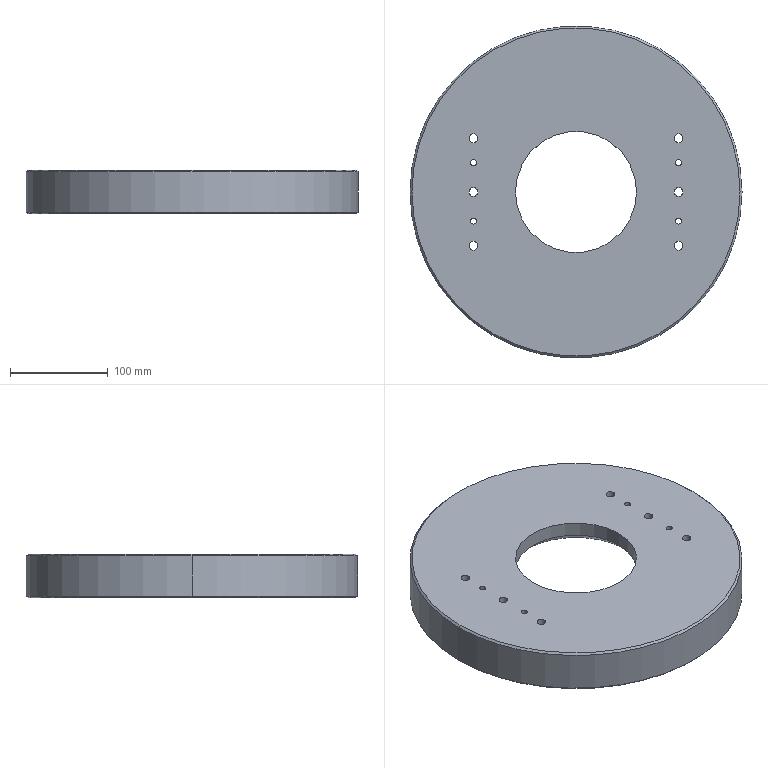NC program | NX | posted with a generic post | part box 340 x 340 x 45 mm
Whole program:
N10 G17 G21 G94 G90
(FLOOR_WALL_COPY , TOOL : D63)
N12 T01 M6
N14 G54
N16 G17 G0 G90 X-114.089 Y169.727 S6500 M3
N18 G43 Z75. H1
N20 Z48.
N22 G94 G1 Z45. F1250.
N24 X-108.622
N26 X108.625
N28 G2 X128.764 Y154.993 R199.71
N30 X136.667 Y148.072 R199.05
N32 X146.571 Y138.275 R199.945
N34 G1 X-146.576
N36 G3 X-149.24 Y135.392 R200.047
N38 X-156.003 Y127.542 R199.804
N40 X-168.04 Y111.199 R198.929
N42 X-170.86 Y106.823 R200.413
N44 G1 X170.865
N46 G2 X179.037 Y92.46 R200.478
N48 X186.882 Y75.372 R200.842
N50 G1 X-186.881
N52 G3 X-192.14 Y60.695 R200.413
N54 G1 X-192.2 Y60.507
N56 G3 X-196.663 Y43.92 R199.967
N58 G1 X196.663
N60 G2 X199.84 Y25.8 R200.842
N62 G1 X199.842 Y25.788
N64 G2 X201.121 Y12.468 R199.892
N66 G1 X-201.117
N68 G3 X-201.5 Y1.732 R199.897
N70 G1 Y-1.795
N72 G3 X-200.607 Y-18.983 R199.897
N74 G1 X200.603
N76 G2 X195.092 Y-50.435 R199.975
N78 G1 X-195.095
N80 G3 X-184.118 Y-81.887 R200.845
N82 G1 X184.122
N84 G2 X168.041 Y-111.199 R200.412
N86 X166.608 Y-113.338 R198.934
N88 G1 X-166.606
N90 G3 X-157.595 Y-125.565 R200.33
N92 X-149.136 Y-135.503 R201.381
N94 X-140.14 Y-144.79 R199.962
N96 G1 X140.149
N98 X144.428
N100 Z48.
N102 G0 Z75.
N104 M5
(ZLEVEL_PROFILE_COPY_1_COPY_COPY_COPY_COPY_2_COPY_COPY_1 , TOOL : D6A45)
N106 T07 M6
N108 G54
N110 G17 G0 G90 X-171.697 Y-1.037 S7000 M3
N112 G43 Z75. H7
N114 Z42.5
N116 G94 G1 X-170.8 Y-0.52 F1000.
N118 G3 X-170.5 Y0. R0.6
N120 G1 Y0.005
N122 G2 X0.005 Y170.5 R170.5
N124 X-170.5 Y0. R-170.5
N126 G3 X-170.8 Y0.52 R0.6
N128 G1 X-171.697 Y1.037
N130 G0 Z75.
(ZLEVEL_PROFILE_COPY_1_COPY_COPY_COPY_COPY_2_COPY_COPY_1_COPY , TOOL : D6A45)
N132 X-58.332 Y1.045
N134 Z42.5
N136 G1 X-59.241 Y0.52
N138 G3 X-59.541 Y0. R0.6
N140 G1 Y-0.008
N142 G3 X0.008 Y-59.541 R59.541
N144 X-59.541 Y0. R-59.541
N146 X-59.241 Y-0.52 R0.6
N148 G1 X-58.332 Y-1.045
N150 G0 Z75.
N152 M5
N154 M2